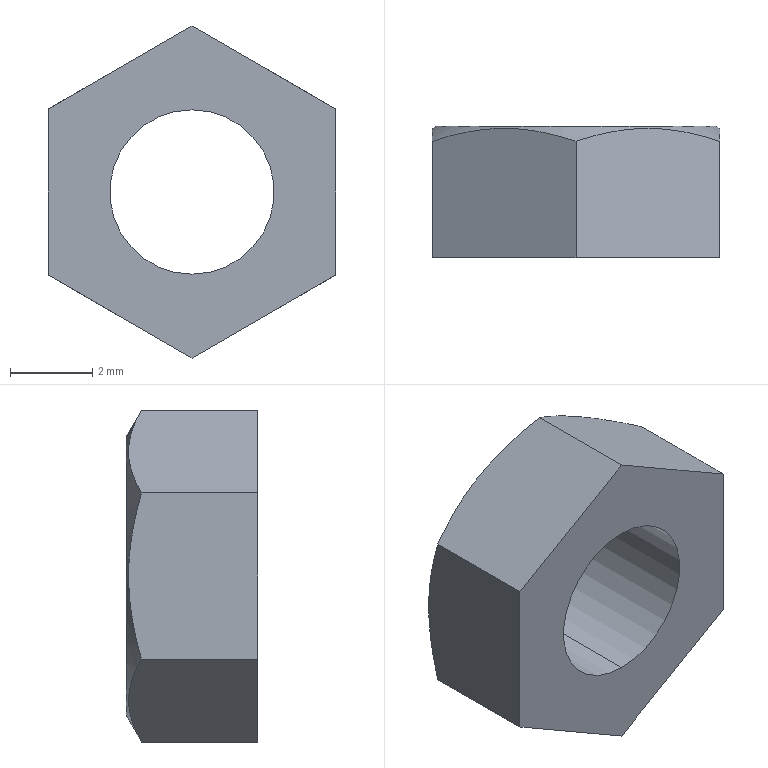Part | STEP file | NN42-M4 | 1 solid | 12 faces | box 7 x 3.2 x 8.083 mm | volume 94.914 mm3 | plane 8 | cylinder 2 | cone 2 | commonest cylinder face diameters 4 x2
STEP:
#1=CARTESIAN_POINT('',(0.,0.,0.));
#2=DIRECTION('',(0.,0.,1.));
#3=DIRECTION('',(1.,0.,0.));
#4=AXIS2_PLACEMENT_3D('',#1,#2,#3);
#5=CARTESIAN_POINT('',(0.,3.2,-2.));
#6=VERTEX_POINT('',#5);
#7=CARTESIAN_POINT('',(0.,0.,-2.));
#8=VERTEX_POINT('',#7);
#9=CARTESIAN_POINT('',(0.,3.2,-2.));
#10=DIRECTION('',(0.,-1.,0.));
#11=VECTOR('',#10,1.);
#12=LINE('',#9,#11);
#13=CARTESIAN_POINT('',(0.,3.2,0.));
#14=DIRECTION('',(0.,-1.,0.));
#15=DIRECTION('',(0.,0.,-1.));
#16=AXIS2_PLACEMENT_3D('',#13,#14,#15);
#17=CYLINDRICAL_SURFACE('',#16,2.);
#18=CARTESIAN_POINT('',(6.283,0.));
#19=DIRECTION('',(0.,1.));
#20=VECTOR('',#19,1.);
#21=LINE('',#18,#20);
#22=(GEOMETRIC_REPRESENTATION_CONTEXT(2)PARAMETRIC_REPRESENTATION_CONTEXT()REPRESENTATION_CONTEXT('',''));
#23=DEFINITIONAL_REPRESENTATION('',(#21),#22);
#24=PCURVE('',#17,#23);
#25=CARTESIAN_POINT('',(0.,3.2,0.));
#26=DIRECTION('',(0.,-1.,0.));
#27=DIRECTION('',(0.,0.,-1.));
#28=AXIS2_PLACEMENT_3D('',#25,#26,#27);
#29=CYLINDRICAL_SURFACE('',#28,2.);
#30=CARTESIAN_POINT('',(0.,0.));
#31=DIRECTION('',(0.,1.));
#32=VECTOR('',#31,1.);
#33=LINE('',#30,#32);
#34=(GEOMETRIC_REPRESENTATION_CONTEXT(2)PARAMETRIC_REPRESENTATION_CONTEXT()REPRESENTATION_CONTEXT('',''));
#35=DEFINITIONAL_REPRESENTATION('',(#33),#34);
#36=PCURVE('',#29,#35);
#37=SURFACE_CURVE('',#12,(#24,#36),.PCURVE_S1.);
#38=EDGE_CURVE('',#6,#8,#37,.T.);
#39=ORIENTED_EDGE('',*,*,#38,.T.);
#40=CARTESIAN_POINT('',(0.,0.,2.));
#41=VERTEX_POINT('',#40);
#42=CARTESIAN_POINT('',(0.,0.,0.));
#43=DIRECTION('',(0.,1.,0.));
#44=DIRECTION('',(0.,0.,1.));
#45=AXIS2_PLACEMENT_3D('',#42,#43,#44);
#46=CIRCLE('',#45,2.);
#47=CARTESIAN_POINT('',(9.425,3.2));
#48=DIRECTION('',(-1.,0.));
#49=VECTOR('',#48,1.);
#50=LINE('',#47,#49);
#51=(GEOMETRIC_REPRESENTATION_CONTEXT(2)PARAMETRIC_REPRESENTATION_CONTEXT()REPRESENTATION_CONTEXT('',''));
#52=DEFINITIONAL_REPRESENTATION('',(#50),#51);
#53=PCURVE('',#17,#52);
#54=CARTESIAN_POINT('',(0.,0.,0.));
#55=DIRECTION('',(0.,-1.,0.));
#56=DIRECTION('',(0.,0.,1.));
#57=AXIS2_PLACEMENT_3D('',#54,#55,#56);
#58=PLANE('',#57);
#59=CARTESIAN_POINT('',(2.,0.));
#60=CARTESIAN_POINT('',(2.,-3.464));
#61=CARTESIAN_POINT('',(-1.,-1.732));
#62=CARTESIAN_POINT('',(-4.,0.));
#63=CARTESIAN_POINT('',(-1.,1.732));
#64=CARTESIAN_POINT('',(2.,3.464));
#65=CARTESIAN_POINT('',(2.,0.));
#66=(BOUNDED_CURVE()B_SPLINE_CURVE(2,(#59,#60,#61,#62,#63,#64,#65),.UNSPECIFIED.,.T.,.F.)B_SPLINE_CURVE_WITH_KNOTS((1,2,2,2,2,1),(-2.094,0.,2.094,4.189,6.283,8.378),.UNSPECIFIED.)CURVE()GEOMETRIC_REPRESENTATION_ITEM()RATIONAL_B_SPLINE_CURVE((1.,0.5,1.,0.5,1.,0.5,1.))REPRESENTATION_ITEM(''));
#67=(GEOMETRIC_REPRESENTATION_CONTEXT(2)PARAMETRIC_REPRESENTATION_CONTEXT()REPRESENTATION_CONTEXT('',''));
#68=DEFINITIONAL_REPRESENTATION('',(#66),#67);
#69=PCURVE('',#58,#68);
#70=SURFACE_CURVE('',#46,(#53,#69),.PCURVE_S1.);
#71=EDGE_CURVE('',#8,#41,#70,.T.);
#72=ORIENTED_EDGE('',*,*,#71,.T.);
#73=CARTESIAN_POINT('',(0.,3.2,2.));
#74=VERTEX_POINT('',#73);
#75=CARTESIAN_POINT('',(0.,3.2,2.));
#76=DIRECTION('',(0.,-1.,0.));
#77=VECTOR('',#76,1.);
#78=LINE('',#75,#77);
#79=CARTESIAN_POINT('',(3.142,0.));
#80=DIRECTION('',(0.,1.));
#81=VECTOR('',#80,1.);
#82=LINE('',#79,#81);
#83=(GEOMETRIC_REPRESENTATION_CONTEXT(2)PARAMETRIC_REPRESENTATION_CONTEXT()REPRESENTATION_CONTEXT('',''));
#84=DEFINITIONAL_REPRESENTATION('',(#82),#83);
#85=PCURVE('',#17,#84);
#86=CARTESIAN_POINT('',(3.142,0.));
#87=DIRECTION('',(0.,1.));
#88=VECTOR('',#87,1.);
#89=LINE('',#86,#88);
#90=(GEOMETRIC_REPRESENTATION_CONTEXT(2)PARAMETRIC_REPRESENTATION_CONTEXT()REPRESENTATION_CONTEXT('',''));
#91=DEFINITIONAL_REPRESENTATION('',(#89),#90);
#92=PCURVE('',#29,#91);
#93=SURFACE_CURVE('',#78,(#85,#92),.PCURVE_S1.);
#94=EDGE_CURVE('',#74,#41,#93,.T.);
#95=ORIENTED_EDGE('',*,*,#94,.F.);
#96=CARTESIAN_POINT('',(0.,3.2,0.));
#97=DIRECTION('',(0.,-1.,0.));
#98=DIRECTION('',(0.,0.,-1.));
#99=AXIS2_PLACEMENT_3D('',#96,#97,#98);
#100=CIRCLE('',#99,2.);
#101=CARTESIAN_POINT('',(0.,0.));
#102=DIRECTION('',(1.,0.));
#103=VECTOR('',#102,1.);
#104=LINE('',#101,#103);
#105=(GEOMETRIC_REPRESENTATION_CONTEXT(2)PARAMETRIC_REPRESENTATION_CONTEXT()REPRESENTATION_CONTEXT('',''));
#106=DEFINITIONAL_REPRESENTATION('',(#104),#105);
#107=PCURVE('',#17,#106);
#108=CARTESIAN_POINT('',(0.,3.2,0.));
#109=DIRECTION('',(0.,1.,0.));
#110=DIRECTION('',(-1.,0.,0.));
#111=AXIS2_PLACEMENT_3D('',#108,#109,#110);
#112=PLANE('',#111);
#113=CARTESIAN_POINT('',(0.,-2.));
#114=CARTESIAN_POINT('',(-3.464,-2.));
#115=CARTESIAN_POINT('',(-1.732,1.));
#116=CARTESIAN_POINT('',(0.,4.));
#117=CARTESIAN_POINT('',(1.732,1.));
#118=CARTESIAN_POINT('',(3.464,-2.));
#119=CARTESIAN_POINT('',(0.,-2.));
#120=(BOUNDED_CURVE()B_SPLINE_CURVE(2,(#113,#114,#115,#116,#117,#118,#119),.UNSPECIFIED.,.T.,.F.)B_SPLINE_CURVE_WITH_KNOTS((1,2,2,2,2,1),(-2.094,0.,2.094,4.189,6.283,8.378),.UNSPECIFIED.)CURVE()GEOMETRIC_REPRESENTATION_ITEM()RATIONAL_B_SPLINE_CURVE((1.,0.5,1.,0.5,1.,0.5,1.))REPRESENTATION_ITEM(''));
#121=(GEOMETRIC_REPRESENTATION_CONTEXT(2)PARAMETRIC_REPRESENTATION_CONTEXT()REPRESENTATION_CONTEXT('',''));
#122=DEFINITIONAL_REPRESENTATION('',(#120),#121);
#123=PCURVE('',#112,#122);
#124=SURFACE_CURVE('',#100,(#107,#123),.PCURVE_S1.);
#125=EDGE_CURVE('',#74,#6,#124,.T.);
#126=ORIENTED_EDGE('',*,*,#125,.T.);
#127=EDGE_LOOP('',(#39,#72,#95,#126));
#128=FACE_BOUND('',#127,.F.);
#129=ADVANCED_FACE('',(#128),#17,.F.);
#130=CARTESIAN_POINT('',(3.4,3.2,0.));
#131=VERTEX_POINT('',#130);
#132=CARTESIAN_POINT('',(-3.4,3.2,0.));
#133=VERTEX_POINT('',#132);
#134=CARTESIAN_POINT('',(0.,3.2,0.));
#135=DIRECTION('',(0.,-1.,0.));
#136=DIRECTION('',(1.,0.,0.));
#137=AXIS2_PLACEMENT_3D('',#134,#135,#136);
#138=CIRCLE('',#137,3.4);
#139=CARTESIAN_POINT('',(0.,3.2,0.));
#140=DIRECTION('',(0.,-1.,0.));
#141=DIRECTION('',(1.,0.,0.));
#142=AXIS2_PLACEMENT_3D('',#139,#140,#141);
#143=CONICAL_SURFACE('',#142,3.4,1.047);
#144=CARTESIAN_POINT('',(0.,0.));
#145=DIRECTION('',(1.,0.));
#146=VECTOR('',#145,1.);
#147=LINE('',#144,#146);
#148=(GEOMETRIC_REPRESENTATION_CONTEXT(2)PARAMETRIC_REPRESENTATION_CONTEXT()REPRESENTATION_CONTEXT('',''));
#149=DEFINITIONAL_REPRESENTATION('',(#147),#148);
#150=PCURVE('',#143,#149);
#151=CARTESIAN_POINT('',(-3.4,0.));
#152=CARTESIAN_POINT('',(-3.4,5.889));
#153=CARTESIAN_POINT('',(1.7,2.944));
#154=CARTESIAN_POINT('',(6.8,0.));
#155=CARTESIAN_POINT('',(1.7,-2.944));
#156=CARTESIAN_POINT('',(-3.4,-5.889));
#157=CARTESIAN_POINT('',(-3.4,0.));
#158=(BOUNDED_CURVE()B_SPLINE_CURVE(2,(#151,#152,#153,#154,#155,#156,#157),.UNSPECIFIED.,.T.,.F.)B_SPLINE_CURVE_WITH_KNOTS((1,2,2,2,2,1),(-2.094,0.,2.094,4.189,6.283,8.378),.UNSPECIFIED.)CURVE()GEOMETRIC_REPRESENTATION_ITEM()RATIONAL_B_SPLINE_CURVE((1.,0.5,1.,0.5,1.,0.5,1.))REPRESENTATION_ITEM(''));
#159=(GEOMETRIC_REPRESENTATION_CONTEXT(2)PARAMETRIC_REPRESENTATION_CONTEXT()REPRESENTATION_CONTEXT('',''));
#160=DEFINITIONAL_REPRESENTATION('',(#158),#159);
#161=PCURVE('',#112,#160);
#162=SURFACE_CURVE('',#138,(#150,#161),.PCURVE_S1.);
#163=EDGE_CURVE('',#131,#133,#162,.T.);
#164=ORIENTED_EDGE('',*,*,#163,.T.);
#165=CARTESIAN_POINT('',(-3.5,3.142,0.));
#166=VERTEX_POINT('',#165);
#167=CARTESIAN_POINT('',(-3.4,3.2,0.));
#168=DIRECTION('',(-0.866,-0.5,0.));
#169=VECTOR('',#168,1.);
#170=LINE('',#167,#169);
#171=CARTESIAN_POINT('',(3.142,0.));
#172=DIRECTION('',(0.,1.));
#173=VECTOR('',#172,1.);
#174=LINE('',#171,#173);
#175=(GEOMETRIC_REPRESENTATION_CONTEXT(2)PARAMETRIC_REPRESENTATION_CONTEXT()REPRESENTATION_CONTEXT('',''));
#176=DEFINITIONAL_REPRESENTATION('',(#174),#175);
#177=PCURVE('',#143,#176);
#178=CARTESIAN_POINT('',(0.,3.2,0.));
#179=DIRECTION('',(0.,-1.,0.));
#180=DIRECTION('',(1.,0.,0.));
#181=AXIS2_PLACEMENT_3D('',#178,#179,#180);
#182=CONICAL_SURFACE('',#181,3.4,1.047);
#183=CARTESIAN_POINT('',(3.142,0.));
#184=DIRECTION('',(0.,1.));
#185=VECTOR('',#184,1.);
#186=LINE('',#183,#185);
#187=(GEOMETRIC_REPRESENTATION_CONTEXT(2)PARAMETRIC_REPRESENTATION_CONTEXT()REPRESENTATION_CONTEXT('',''));
#188=DEFINITIONAL_REPRESENTATION('',(#186),#187);
#189=PCURVE('',#182,#188);
#190=SURFACE_CURVE('',#170,(#177,#189),.PCURVE_S1.);
#191=EDGE_CURVE('',#133,#166,#190,.T.);
#192=ORIENTED_EDGE('',*,*,#191,.T.);
#193=CARTESIAN_POINT('',(-3.5,2.83,2.021));
#194=VERTEX_POINT('',#193);
#195=CARTESIAN_POINT('',(-3.5,2.83,2.021));
#196=CARTESIAN_POINT('',(-3.5,3.02,1.362));
#197=CARTESIAN_POINT('',(-3.5,3.142,0.6921));
#198=CARTESIAN_POINT('',(-3.5,3.142,0.));
#199=B_SPLINE_CURVE_WITH_KNOTS('',3,(#195,#196,#197,#198),.UNSPECIFIED.,.F.,.F.,(4,4),(0.004408,0.006464),.PIECEWISE_BEZIER_KNOTS.);
#200=CARTESIAN_POINT('',(2.618,0.3703));
#201=CARTESIAN_POINT('',(2.624,0.3617));
#202=CARTESIAN_POINT('',(2.637,0.3447));
#203=CARTESIAN_POINT('',(2.657,0.3201));
#204=CARTESIAN_POINT('',(2.678,0.2963));
#205=CARTESIAN_POINT('',(2.699,0.2735));
#206=CARTESIAN_POINT('',(2.72,0.2516));
#207=CARTESIAN_POINT('',(2.742,0.2307));
#208=CARTESIAN_POINT('',(2.764,0.2108));
#209=CARTESIAN_POINT('',(2.787,0.192));
#210=CARTESIAN_POINT('',(2.81,0.1743));
#211=CARTESIAN_POINT('',(2.833,0.1577));
#212=CARTESIAN_POINT('',(2.857,0.1422));
#213=CARTESIAN_POINT('',(2.882,0.1279));
#214=CARTESIAN_POINT('',(2.906,0.1149));
#215=CARTESIAN_POINT('',(2.931,0.1031));
#216=CARTESIAN_POINT('',(2.957,0.09264));
#217=CARTESIAN_POINT('',(2.982,0.08345));
#218=CARTESIAN_POINT('',(3.008,0.07562));
#219=CARTESIAN_POINT('',(3.035,0.06915));
#220=CARTESIAN_POINT('',(3.061,0.06408));
#221=CARTESIAN_POINT('',(3.088,0.06043));
#222=CARTESIAN_POINT('',(3.115,0.05823));
#223=CARTESIAN_POINT('',(3.133,0.05773));
#224=CARTESIAN_POINT('',(3.142,0.05774));
#225=B_SPLINE_CURVE_WITH_KNOTS('',3,(#200,#201,#202,#203,#204,#205,#206,#207,#208,#209,#210,#211,#212,#213,#214,#215,#216,#217,#218,#219,#220,#221,#222,#223,#224),.UNSPECIFIED.,.F.,.F.,(4,1,1,1,1,1,1,1,1,1,1,1,1,1,1,1,1,1,1,1,1,1,4),(0.004408,0.004502,0.004595,0.004689,0.004782,0.004875,0.004969,0.005062,0.005156,0.005249,0.005343,0.005436,0.00553,0.005623,0.005716,0.00581,0.005903,0.005997,0.00609,0.006184,0.006277,0.006371,0.006464),.QUASI_UNIFORM_KNOTS.);
#226=(GEOMETRIC_REPRESENTATION_CONTEXT(2)PARAMETRIC_REPRESENTATION_CONTEXT()REPRESENTATION_CONTEXT('',''));
#227=DEFINITIONAL_REPRESENTATION('',(#225),#226);
#228=PCURVE('',#143,#227);
#229=CARTESIAN_POINT('',(-3.5,2.83,2.021));
#230=DIRECTION('',(1.,0.,0.));
#231=DIRECTION('',(0.,0.,1.));
#232=AXIS2_PLACEMENT_3D('',#229,#230,#231);
#233=PLANE('',#232);
#234=CARTESIAN_POINT('',(0.,0.));
#235=CARTESIAN_POINT('',(-0.6583,-0.19));
#236=CARTESIAN_POINT('',(-1.329,-0.3126));
#237=CARTESIAN_POINT('',(-2.021,-0.3126));
#238=B_SPLINE_CURVE_WITH_KNOTS('',3,(#234,#235,#236,#237),.UNSPECIFIED.,.F.,.F.,(4,4),(0.004408,0.006464),.PIECEWISE_BEZIER_KNOTS.);
#239=(GEOMETRIC_REPRESENTATION_CONTEXT(2)PARAMETRIC_REPRESENTATION_CONTEXT()REPRESENTATION_CONTEXT('',''));
#240=DEFINITIONAL_REPRESENTATION('',(#238),#239);
#241=PCURVE('',#233,#240);
#242=SURFACE_CURVE('',#199,(#228,#241),.PCURVE_S1.);
#243=EDGE_CURVE('',#194,#166,#242,.T.);
#244=ORIENTED_EDGE('',*,*,#243,.F.);
#245=CARTESIAN_POINT('',(0.,2.83,4.041));
#246=VERTEX_POINT('',#245);
#247=CARTESIAN_POINT('',(0.,2.83,4.041));
#248=CARTESIAN_POINT('',(-0.5715,3.02,3.712));
#249=CARTESIAN_POINT('',(-1.152,3.142,3.377));
#250=CARTESIAN_POINT('',(-2.044,3.142,2.861));
#251=CARTESIAN_POINT('',(-2.341,3.113,2.69));
#252=CARTESIAN_POINT('',(-2.925,3.004,2.352));
#253=CARTESIAN_POINT('',(-3.214,2.925,2.186));
#254=CARTESIAN_POINT('',(-3.5,2.83,2.021));
#255=B_SPLINE_CURVE_WITH_KNOTS('',3,(#247,#248,#249,#250,#251,#252,#253,#254),.UNSPECIFIED.,.F.,.F.,(4,2,2,4),(0.000000238,0.002041,0.003061,0.004082),.UNSPECIFIED.);
#256=CARTESIAN_POINT('',(1.571,0.3703));
#257=CARTESIAN_POINT('',(1.584,0.353));
#258=CARTESIAN_POINT('',(1.61,0.3195));
#259=CARTESIAN_POINT('',(1.651,0.2728));
#260=CARTESIAN_POINT('',(1.694,0.23));
#261=CARTESIAN_POINT('',(1.739,0.1913));
#262=CARTESIAN_POINT('',(1.786,0.157));
#263=CARTESIAN_POINT('',(1.834,0.1273));
#264=CARTESIAN_POINT('',(1.884,0.1025));
#265=CARTESIAN_POINT('',(1.935,0.08287));
#266=CARTESIAN_POINT('',(1.987,0.06856));
#267=CARTESIAN_POINT('',(2.04,0.05981));
#268=CARTESIAN_POINT('',(2.093,0.05676));
#269=CARTESIAN_POINT('',(2.147,0.05956));
#270=CARTESIAN_POINT('',(2.2,0.06812));
#271=CARTESIAN_POINT('',(2.252,0.08231));
#272=CARTESIAN_POINT('',(2.304,0.1019));
#273=CARTESIAN_POINT('',(2.354,0.1267));
#274=CARTESIAN_POINT('',(2.402,0.1565));
#275=CARTESIAN_POINT('',(2.449,0.1909));
#276=CARTESIAN_POINT('',(2.494,0.2297));
#277=CARTESIAN_POINT('',(2.537,0.2726));
#278=CARTESIAN_POINT('',(2.579,0.3194));
#279=CARTESIAN_POINT('',(2.605,0.353));
#280=CARTESIAN_POINT('',(2.618,0.3703));
#281=B_SPLINE_CURVE_WITH_KNOTS('',3,(#256,#257,#258,#259,#260,#261,#262,#263,#264,#265,#266,#267,#268,#269,#270,#271,#272,#273,#274,#275,#276,#277,#278,#279,#280),.UNSPECIFIED.,.F.,.F.,(4,1,1,1,1,1,1,1,1,1,1,1,1,1,1,1,1,1,1,1,1,1,4),(0.000000238,0.0001858,0.0003713,0.0005568,0.0007424,0.0009279,0.001113,0.001299,0.001484,0.00167,0.001856,0.002041,0.002227,0.002412,0.002598,0.002783,0.002969,0.003154,0.00334,0.003525,0.003711,0.003896,0.004082),.QUASI_UNIFORM_KNOTS.);
#282=(GEOMETRIC_REPRESENTATION_CONTEXT(2)PARAMETRIC_REPRESENTATION_CONTEXT()REPRESENTATION_CONTEXT('',''));
#283=DEFINITIONAL_REPRESENTATION('',(#281),#282);
#284=PCURVE('',#143,#283);
#285=CARTESIAN_POINT('',(0.,2.83,4.041));
#286=DIRECTION('',(0.5,0.,-0.866));
#287=DIRECTION('',(0.866,0.,0.5));
#288=AXIS2_PLACEMENT_3D('',#285,#286,#287);
#289=PLANE('',#288);
#290=CARTESIAN_POINT('',(0.,0.));
#291=CARTESIAN_POINT('',(-0.6599,-0.1905));
#292=CARTESIAN_POINT('',(-1.33,-0.3122));
#293=CARTESIAN_POINT('',(-2.36,-0.3128));
#294=CARTESIAN_POINT('',(-2.704,-0.283));
#295=CARTESIAN_POINT('',(-3.378,-0.1741));
#296=CARTESIAN_POINT('',(-3.711,-0.09537));
#297=CARTESIAN_POINT('',(-4.041,0.));
#298=B_SPLINE_CURVE_WITH_KNOTS('',3,(#290,#291,#292,#293,#294,#295,#296,#297),.UNSPECIFIED.,.F.,.F.,(4,2,2,4),(0.000000238,0.002041,0.003061,0.004082),.UNSPECIFIED.);
#299=(GEOMETRIC_REPRESENTATION_CONTEXT(2)PARAMETRIC_REPRESENTATION_CONTEXT()REPRESENTATION_CONTEXT('',''));
#300=DEFINITIONAL_REPRESENTATION('',(#298),#299);
#301=PCURVE('',#289,#300);
#302=SURFACE_CURVE('',#255,(#284,#301),.PCURVE_S1.);
#303=EDGE_CURVE('',#246,#194,#302,.T.);
#304=ORIENTED_EDGE('',*,*,#303,.F.);
#305=CARTESIAN_POINT('',(3.5,2.83,2.021));
#306=VERTEX_POINT('',#305);
#307=CARTESIAN_POINT('',(3.5,2.83,2.021));
#308=CARTESIAN_POINT('',(2.929,3.02,2.351));
#309=CARTESIAN_POINT('',(2.348,3.142,2.686));
#310=CARTESIAN_POINT('',(1.456,3.142,3.201));
#311=CARTESIAN_POINT('',(1.159,3.113,3.373));
#312=CARTESIAN_POINT('',(0.5746,3.004,3.71));
#313=CARTESIAN_POINT('',(0.2861,2.925,3.876));
#314=CARTESIAN_POINT('',(0.,2.83,4.041));
#315=B_SPLINE_CURVE_WITH_KNOTS('',3,(#307,#308,#309,#310,#311,#312,#313,#314),.UNSPECIFIED.,.F.,.F.,(4,2,2,4),(0.000000238,0.002041,0.003061,0.004082),.UNSPECIFIED.);
#316=CARTESIAN_POINT('',(0.5236,0.3703));
#317=CARTESIAN_POINT('',(0.5365,0.353));
#318=CARTESIAN_POINT('',(0.5628,0.3195));
#319=CARTESIAN_POINT('',(0.6041,0.2728));
#320=CARTESIAN_POINT('',(0.6472,0.23));
#321=CARTESIAN_POINT('',(0.6921,0.1913));
#322=CARTESIAN_POINT('',(0.7388,0.157));
#323=CARTESIAN_POINT('',(0.787,0.1273));
#324=CARTESIAN_POINT('',(0.8367,0.1025));
#325=CARTESIAN_POINT('',(0.8877,0.08287));
#326=CARTESIAN_POINT('',(0.9398,0.06856));
#327=CARTESIAN_POINT('',(0.9926,0.05981));
#328=CARTESIAN_POINT('',(1.046,0.05676));
#329=CARTESIAN_POINT('',(1.1,0.05956));
#330=CARTESIAN_POINT('',(1.153,0.06812));
#331=CARTESIAN_POINT('',(1.205,0.08231));
#332=CARTESIAN_POINT('',(1.257,0.1019));
#333=CARTESIAN_POINT('',(1.307,0.1267));
#334=CARTESIAN_POINT('',(1.355,0.1565));
#335=CARTESIAN_POINT('',(1.402,0.1909));
#336=CARTESIAN_POINT('',(1.447,0.2297));
#337=CARTESIAN_POINT('',(1.49,0.2726));
#338=CARTESIAN_POINT('',(1.532,0.3194));
#339=CARTESIAN_POINT('',(1.558,0.353));
#340=CARTESIAN_POINT('',(1.571,0.3703));
#341=B_SPLINE_CURVE_WITH_KNOTS('',3,(#316,#317,#318,#319,#320,#321,#322,#323,#324,#325,#326,#327,#328,#329,#330,#331,#332,#333,#334,#335,#336,#337,#338,#339,#340),.UNSPECIFIED.,.F.,.F.,(4,1,1,1,1,1,1,1,1,1,1,1,1,1,1,1,1,1,1,1,1,1,4),(0.000000238,0.0001858,0.0003713,0.0005568,0.0007424,0.0009279,0.001113,0.001299,0.001484,0.00167,0.001856,0.002041,0.002227,0.002412,0.002598,0.002783,0.002969,0.003154,0.00334,0.003525,0.003711,0.003896,0.004082),.QUASI_UNIFORM_KNOTS.);
#342=(GEOMETRIC_REPRESENTATION_CONTEXT(2)PARAMETRIC_REPRESENTATION_CONTEXT()REPRESENTATION_CONTEXT('',''));
#343=DEFINITIONAL_REPRESENTATION('',(#341),#342);
#344=PCURVE('',#143,#343);
#345=CARTESIAN_POINT('',(3.5,2.83,2.021));
#346=DIRECTION('',(-0.5,0.,-0.866));
#347=DIRECTION('',(0.866,0.,-0.5));
#348=AXIS2_PLACEMENT_3D('',#345,#346,#347);
#349=PLANE('',#348);
#350=CARTESIAN_POINT('',(0.,0.));
#351=CARTESIAN_POINT('',(-0.6599,-0.1905));
#352=CARTESIAN_POINT('',(-1.33,-0.3122));
#353=CARTESIAN_POINT('',(-2.36,-0.3128));
#354=CARTESIAN_POINT('',(-2.704,-0.283));
#355=CARTESIAN_POINT('',(-3.378,-0.1741));
#356=CARTESIAN_POINT('',(-3.711,-0.09537));
#357=CARTESIAN_POINT('',(-4.041,0.));
#358=B_SPLINE_CURVE_WITH_KNOTS('',3,(#350,#351,#352,#353,#354,#355,#356,#357),.UNSPECIFIED.,.F.,.F.,(4,2,2,4),(0.000000238,0.002041,0.003061,0.004082),.UNSPECIFIED.);
#359=(GEOMETRIC_REPRESENTATION_CONTEXT(2)PARAMETRIC_REPRESENTATION_CONTEXT()REPRESENTATION_CONTEXT('',''));
#360=DEFINITIONAL_REPRESENTATION('',(#358),#359);
#361=PCURVE('',#349,#360);
#362=SURFACE_CURVE('',#315,(#344,#361),.PCURVE_S1.);
#363=EDGE_CURVE('',#306,#246,#362,.T.);
#364=ORIENTED_EDGE('',*,*,#363,.F.);
#365=CARTESIAN_POINT('',(3.5,3.142,0.));
#366=VERTEX_POINT('',#365);
#367=CARTESIAN_POINT('',(3.5,3.142,0.));
#368=CARTESIAN_POINT('',(3.5,3.142,0.6917));
#369=CARTESIAN_POINT('',(3.5,3.019,1.363));
#370=CARTESIAN_POINT('',(3.5,2.83,2.021));
#371=B_SPLINE_CURVE_WITH_KNOTS('',3,(#367,#368,#369,#370),.UNSPECIFIED.,.F.,.F.,(4,4),(0.006464,0.008519),.PIECEWISE_BEZIER_KNOTS.);
#372=CARTESIAN_POINT('',(0.,0.05774));
#373=CARTESIAN_POINT('',(0.008983,0.05773));
#374=CARTESIAN_POINT('',(0.02693,0.05823));
#375=CARTESIAN_POINT('',(0.05373,0.06043));
#376=CARTESIAN_POINT('',(0.08039,0.06408));
#377=CARTESIAN_POINT('',(0.1069,0.06915));
#378=CARTESIAN_POINT('',(0.1331,0.07562));
#379=CARTESIAN_POINT('',(0.1591,0.08346));
#380=CARTESIAN_POINT('',(0.1849,0.09265));
#381=CARTESIAN_POINT('',(0.2103,0.1031));
#382=CARTESIAN_POINT('',(0.2354,0.1149));
#383=CARTESIAN_POINT('',(0.2601,0.128));
#384=CARTESIAN_POINT('',(0.2845,0.1422));
#385=CARTESIAN_POINT('',(0.3084,0.1577));
#386=CARTESIAN_POINT('',(0.332,0.1743));
#387=CARTESIAN_POINT('',(0.3551,0.1921));
#388=CARTESIAN_POINT('',(0.3778,0.2109));
#389=CARTESIAN_POINT('',(0.4,0.2308));
#390=CARTESIAN_POINT('',(0.4218,0.2516));
#391=CARTESIAN_POINT('',(0.4431,0.2735));
#392=CARTESIAN_POINT('',(0.4639,0.2964));
#393=CARTESIAN_POINT('',(0.4843,0.3201));
#394=CARTESIAN_POINT('',(0.5042,0.3447));
#395=CARTESIAN_POINT('',(0.5172,0.3617));
#396=CARTESIAN_POINT('',(0.5236,0.3703));
#397=B_SPLINE_CURVE_WITH_KNOTS('',3,(#372,#373,#374,#375,#376,#377,#378,#379,#380,#381,#382,#383,#384,#385,#386,#387,#388,#389,#390,#391,#392,#393,#394,#395,#396),.UNSPECIFIED.,.F.,.F.,(4,1,1,1,1,1,1,1,1,1,1,1,1,1,1,1,1,1,1,1,1,1,4),(0.006464,0.006557,0.006651,0.006744,0.006838,0.006931,0.007024,0.007118,0.007211,0.007305,0.007398,0.007491,0.007585,0.007678,0.007772,0.007865,0.007958,0.008052,0.008145,0.008239,0.008332,0.008425,0.008519),.QUASI_UNIFORM_KNOTS.);
#398=(GEOMETRIC_REPRESENTATION_CONTEXT(2)PARAMETRIC_REPRESENTATION_CONTEXT()REPRESENTATION_CONTEXT('',''));
#399=DEFINITIONAL_REPRESENTATION('',(#397),#398);
#400=PCURVE('',#143,#399);
#401=CARTESIAN_POINT('',(3.5,2.83,-2.021));
#402=DIRECTION('',(-1.,0.,0.));
#403=DIRECTION('',(0.,0.,-1.));
#404=AXIS2_PLACEMENT_3D('',#401,#402,#403);
#405=PLANE('',#404);
#406=CARTESIAN_POINT('',(-2.021,-0.3126));
#407=CARTESIAN_POINT('',(-2.712,-0.3126));
#408=CARTESIAN_POINT('',(-3.384,-0.1898));
#409=CARTESIAN_POINT('',(-4.041,0.));
#410=B_SPLINE_CURVE_WITH_KNOTS('',3,(#406,#407,#408,#409),.UNSPECIFIED.,.F.,.F.,(4,4),(0.006464,0.008519),.PIECEWISE_BEZIER_KNOTS.);
#411=(GEOMETRIC_REPRESENTATION_CONTEXT(2)PARAMETRIC_REPRESENTATION_CONTEXT()REPRESENTATION_CONTEXT('',''));
#412=DEFINITIONAL_REPRESENTATION('',(#410),#411);
#413=PCURVE('',#405,#412);
#414=SURFACE_CURVE('',#371,(#400,#413),.PCURVE_S1.);
#415=EDGE_CURVE('',#366,#306,#414,.T.);
#416=ORIENTED_EDGE('',*,*,#415,.F.);
#417=CARTESIAN_POINT('',(3.4,3.2,0.));
#418=DIRECTION('',(0.866,-0.5,0.));
#419=VECTOR('',#418,1.);
#420=LINE('',#417,#419);
#421=CARTESIAN_POINT('',(0.,0.));
#422=DIRECTION('',(0.,1.));
#423=VECTOR('',#422,1.);
#424=LINE('',#421,#423);
#425=(GEOMETRIC_REPRESENTATION_CONTEXT(2)PARAMETRIC_REPRESENTATION_CONTEXT()REPRESENTATION_CONTEXT('',''));
#426=DEFINITIONAL_REPRESENTATION('',(#424),#425);
#427=PCURVE('',#143,#426);
#428=CARTESIAN_POINT('',(6.283,0.));
#429=DIRECTION('',(0.,1.));
#430=VECTOR('',#429,1.);
#431=LINE('',#428,#430);
#432=(GEOMETRIC_REPRESENTATION_CONTEXT(2)PARAMETRIC_REPRESENTATION_CONTEXT()REPRESENTATION_CONTEXT('',''));
#433=DEFINITIONAL_REPRESENTATION('',(#431),#432);
#434=PCURVE('',#182,#433);
#435=SURFACE_CURVE('',#420,(#427,#434),.PCURVE_S1.);
#436=EDGE_CURVE('',#131,#366,#435,.T.);
#437=ORIENTED_EDGE('',*,*,#436,.F.);
#438=EDGE_LOOP('',(#164,#192,#244,#304,#364,#416,#437));
#439=FACE_BOUND('',#438,.T.);
#440=ADVANCED_FACE('',(#439),#143,.T.);
#441=ORIENTED_EDGE('',*,*,#191,.F.);
#442=CARTESIAN_POINT('',(0.,3.2,0.));
#443=DIRECTION('',(0.,-1.,0.));
#444=DIRECTION('',(1.,0.,0.));
#445=AXIS2_PLACEMENT_3D('',#442,#443,#444);
#446=CIRCLE('',#445,3.4);
#447=CARTESIAN_POINT('',(0.,0.));
#448=DIRECTION('',(1.,0.));
#449=VECTOR('',#448,1.);
#450=LINE('',#447,#449);
#451=(GEOMETRIC_REPRESENTATION_CONTEXT(2)PARAMETRIC_REPRESENTATION_CONTEXT()REPRESENTATION_CONTEXT('',''));
#452=DEFINITIONAL_REPRESENTATION('',(#450),#451);
#453=PCURVE('',#182,#452);
#454=CARTESIAN_POINT('',(-3.4,0.));
#455=CARTESIAN_POINT('',(-3.4,5.889));
#456=CARTESIAN_POINT('',(1.7,2.944));
#457=CARTESIAN_POINT('',(6.8,0.));
#458=CARTESIAN_POINT('',(1.7,-2.944));
#459=CARTESIAN_POINT('',(-3.4,-5.889));
#460=CARTESIAN_POINT('',(-3.4,0.));
#461=(BOUNDED_CURVE()B_SPLINE_CURVE(2,(#454,#455,#456,#457,#458,#459,#460),.UNSPECIFIED.,.T.,.F.)B_SPLINE_CURVE_WITH_KNOTS((1,2,2,2,2,1),(-2.094,0.,2.094,4.189,6.283,8.378),.UNSPECIFIED.)CURVE()GEOMETRIC_REPRESENTATION_ITEM()RATIONAL_B_SPLINE_CURVE((1.,0.5,1.,0.5,1.,0.5,1.))REPRESENTATION_ITEM(''));
#462=(GEOMETRIC_REPRESENTATION_CONTEXT(2)PARAMETRIC_REPRESENTATION_CONTEXT()REPRESENTATION_CONTEXT('',''));
#463=DEFINITIONAL_REPRESENTATION('',(#461),#462);
#464=PCURVE('',#112,#463);
#465=SURFACE_CURVE('',#446,(#453,#464),.PCURVE_S1.);
#466=EDGE_CURVE('',#133,#131,#465,.T.);
#467=ORIENTED_EDGE('',*,*,#466,.T.);
#468=ORIENTED_EDGE('',*,*,#436,.T.);
#469=CARTESIAN_POINT('',(3.5,2.83,-2.021));
#470=VERTEX_POINT('',#469);
#471=CARTESIAN_POINT('',(3.5,2.83,-2.021));
#472=CARTESIAN_POINT('',(3.5,3.02,-1.362));
#473=CARTESIAN_POINT('',(3.5,3.142,-0.6921));
#474=CARTESIAN_POINT('',(3.5,3.142,0.));
#475=B_SPLINE_CURVE_WITH_KNOTS('',3,(#471,#472,#473,#474),.UNSPECIFIED.,.F.,.F.,(4,4),(0.004408,0.006464),.PIECEWISE_BEZIER_KNOTS.);
#476=CARTESIAN_POINT('',(5.76,0.3703));
#477=CARTESIAN_POINT('',(5.766,0.3617));
#478=CARTESIAN_POINT('',(5.779,0.3447));
#479=CARTESIAN_POINT('',(5.799,0.3201));
#480=CARTESIAN_POINT('',(5.819,0.2963));
#481=CARTESIAN_POINT('',(5.84,0.2735));
#482=CARTESIAN_POINT('',(5.861,0.2516));
#483=CARTESIAN_POINT('',(5.883,0.2307));
#484=CARTESIAN_POINT('',(5.905,0.2108));
#485=CARTESIAN_POINT('',(5.928,0.192));
#486=CARTESIAN_POINT('',(5.951,0.1743));
#487=CARTESIAN_POINT('',(5.975,0.1577));
#488=CARTESIAN_POINT('',(5.999,0.1422));
#489=CARTESIAN_POINT('',(6.023,0.1279));
#490=CARTESIAN_POINT('',(6.048,0.1149));
#491=CARTESIAN_POINT('',(6.073,0.1031));
#492=CARTESIAN_POINT('',(6.098,0.09264));
#493=CARTESIAN_POINT('',(6.124,0.08345));
#494=CARTESIAN_POINT('',(6.15,0.07562));
#495=CARTESIAN_POINT('',(6.176,0.06915));
#496=CARTESIAN_POINT('',(6.203,0.06408));
#497=CARTESIAN_POINT('',(6.229,0.06043));
#498=CARTESIAN_POINT('',(6.256,0.05823));
#499=CARTESIAN_POINT('',(6.274,0.05773));
#500=CARTESIAN_POINT('',(6.283,0.05774));
#501=B_SPLINE_CURVE_WITH_KNOTS('',3,(#476,#477,#478,#479,#480,#481,#482,#483,#484,#485,#486,#487,#488,#489,#490,#491,#492,#493,#494,#495,#496,#497,#498,#499,#500),.UNSPECIFIED.,.F.,.F.,(4,1,1,1,1,1,1,1,1,1,1,1,1,1,1,1,1,1,1,1,1,1,4),(0.004408,0.004502,0.004595,0.004689,0.004782,0.004875,0.004969,0.005062,0.005156,0.005249,0.005343,0.005436,0.00553,0.005623,0.005716,0.00581,0.005903,0.005997,0.00609,0.006184,0.006277,0.006371,0.006464),.QUASI_UNIFORM_KNOTS.);
#502=(GEOMETRIC_REPRESENTATION_CONTEXT(2)PARAMETRIC_REPRESENTATION_CONTEXT()REPRESENTATION_CONTEXT('',''));
#503=DEFINITIONAL_REPRESENTATION('',(#501),#502);
#504=PCURVE('',#182,#503);
#505=CARTESIAN_POINT('',(0.,0.));
#506=CARTESIAN_POINT('',(-0.6583,-0.19));
#507=CARTESIAN_POINT('',(-1.329,-0.3126));
#508=CARTESIAN_POINT('',(-2.021,-0.3126));
#509=B_SPLINE_CURVE_WITH_KNOTS('',3,(#505,#506,#507,#508),.UNSPECIFIED.,.F.,.F.,(4,4),(0.004408,0.006464),.PIECEWISE_BEZIER_KNOTS.);
#510=(GEOMETRIC_REPRESENTATION_CONTEXT(2)PARAMETRIC_REPRESENTATION_CONTEXT()REPRESENTATION_CONTEXT('',''));
#511=DEFINITIONAL_REPRESENTATION('',(#509),#510);
#512=PCURVE('',#405,#511);
#513=SURFACE_CURVE('',#475,(#504,#512),.PCURVE_S1.);
#514=EDGE_CURVE('',#470,#366,#513,.T.);
#515=ORIENTED_EDGE('',*,*,#514,.F.);
#516=CARTESIAN_POINT('',(0.,2.83,-4.041));
#517=VERTEX_POINT('',#516);
#518=CARTESIAN_POINT('',(0.,2.83,-4.041));
#519=CARTESIAN_POINT('',(0.5715,3.02,-3.712));
#520=CARTESIAN_POINT('',(1.152,3.142,-3.377));
#521=CARTESIAN_POINT('',(2.044,3.142,-2.861));
#522=CARTESIAN_POINT('',(2.341,3.113,-2.69));
#523=CARTESIAN_POINT('',(2.925,3.004,-2.352));
#524=CARTESIAN_POINT('',(3.214,2.925,-2.186));
#525=CARTESIAN_POINT('',(3.5,2.83,-2.021));
#526=B_SPLINE_CURVE_WITH_KNOTS('',3,(#518,#519,#520,#521,#522,#523,#524,#525),.UNSPECIFIED.,.F.,.F.,(4,2,2,4),(0.000000238,0.002041,0.003061,0.004082),.UNSPECIFIED.);
#527=CARTESIAN_POINT('',(4.712,0.3703));
#528=CARTESIAN_POINT('',(4.725,0.353));
#529=CARTESIAN_POINT('',(4.752,0.3195));
#530=CARTESIAN_POINT('',(4.793,0.2728));
#531=CARTESIAN_POINT('',(4.836,0.23));
#532=CARTESIAN_POINT('',(4.881,0.1913));
#533=CARTESIAN_POINT('',(4.928,0.157));
#534=CARTESIAN_POINT('',(4.976,0.1273));
#535=CARTESIAN_POINT('',(5.026,0.1025));
#536=CARTESIAN_POINT('',(5.076,0.08287));
#537=CARTESIAN_POINT('',(5.129,0.06856));
#538=CARTESIAN_POINT('',(5.181,0.05981));
#539=CARTESIAN_POINT('',(5.235,0.05676));
#540=CARTESIAN_POINT('',(5.288,0.05956));
#541=CARTESIAN_POINT('',(5.342,0.06812));
#542=CARTESIAN_POINT('',(5.394,0.08231));
#543=CARTESIAN_POINT('',(5.445,0.1019));
#544=CARTESIAN_POINT('',(5.495,0.1267));
#545=CARTESIAN_POINT('',(5.544,0.1565));
#546=CARTESIAN_POINT('',(5.591,0.1909));
#547=CARTESIAN_POINT('',(5.636,0.2297));
#548=CARTESIAN_POINT('',(5.679,0.2726));
#549=CARTESIAN_POINT('',(5.72,0.3194));
#550=CARTESIAN_POINT('',(5.747,0.353));
#551=CARTESIAN_POINT('',(5.76,0.3703));
#552=B_SPLINE_CURVE_WITH_KNOTS('',3,(#527,#528,#529,#530,#531,#532,#533,#534,#535,#536,#537,#538,#539,#540,#541,#542,#543,#544,#545,#546,#547,#548,#549,#550,#551),.UNSPECIFIED.,.F.,.F.,(4,1,1,1,1,1,1,1,1,1,1,1,1,1,1,1,1,1,1,1,1,1,4),(0.000000238,0.0001858,0.0003713,0.0005568,0.0007424,0.0009279,0.001113,0.001299,0.001484,0.00167,0.001856,0.002041,0.002227,0.002412,0.002598,0.002783,0.002969,0.003154,0.00334,0.003525,0.003711,0.003896,0.004082),.QUASI_UNIFORM_KNOTS.);
#553=(GEOMETRIC_REPRESENTATION_CONTEXT(2)PARAMETRIC_REPRESENTATION_CONTEXT()REPRESENTATION_CONTEXT('',''));
#554=DEFINITIONAL_REPRESENTATION('',(#552),#553);
#555=PCURVE('',#182,#554);
#556=CARTESIAN_POINT('',(0.,2.83,-4.041));
#557=DIRECTION('',(-0.5,0.,0.866));
#558=DIRECTION('',(-0.866,0.,-0.5));
#559=AXIS2_PLACEMENT_3D('',#556,#557,#558);
#560=PLANE('',#559);
#561=CARTESIAN_POINT('',(0.,0.));
#562=CARTESIAN_POINT('',(-0.6599,-0.1905));
#563=CARTESIAN_POINT('',(-1.33,-0.3122));
#564=CARTESIAN_POINT('',(-2.36,-0.3128));
#565=CARTESIAN_POINT('',(-2.704,-0.283));
#566=CARTESIAN_POINT('',(-3.378,-0.1741));
#567=CARTESIAN_POINT('',(-3.711,-0.09537));
#568=CARTESIAN_POINT('',(-4.041,0.));
#569=B_SPLINE_CURVE_WITH_KNOTS('',3,(#561,#562,#563,#564,#565,#566,#567,#568),.UNSPECIFIED.,.F.,.F.,(4,2,2,4),(0.000000238,0.002041,0.003061,0.004082),.UNSPECIFIED.);
#570=(GEOMETRIC_REPRESENTATION_CONTEXT(2)PARAMETRIC_REPRESENTATION_CONTEXT()REPRESENTATION_CONTEXT('',''));
#571=DEFINITIONAL_REPRESENTATION('',(#569),#570);
#572=PCURVE('',#560,#571);
#573=SURFACE_CURVE('',#526,(#555,#572),.PCURVE_S1.);
#574=EDGE_CURVE('',#517,#470,#573,.T.);
#575=ORIENTED_EDGE('',*,*,#574,.F.);
#576=CARTESIAN_POINT('',(-3.5,2.83,-2.021));
#577=VERTEX_POINT('',#576);
#578=CARTESIAN_POINT('',(-3.5,2.83,-2.021));
#579=CARTESIAN_POINT('',(-2.929,3.02,-2.351));
#580=CARTESIAN_POINT('',(-2.348,3.142,-2.686));
#581=CARTESIAN_POINT('',(-1.456,3.142,-3.201));
#582=CARTESIAN_POINT('',(-1.159,3.113,-3.373));
#583=CARTESIAN_POINT('',(-0.5746,3.004,-3.71));
#584=CARTESIAN_POINT('',(-0.2861,2.925,-3.876));
#585=CARTESIAN_POINT('',(0.,2.83,-4.041));
#586=B_SPLINE_CURVE_WITH_KNOTS('',3,(#578,#579,#580,#581,#582,#583,#584,#585),.UNSPECIFIED.,.F.,.F.,(4,2,2,4),(0.000000238,0.002041,0.003061,0.004082),.UNSPECIFIED.);
#587=CARTESIAN_POINT('',(3.665,0.3703));
#588=CARTESIAN_POINT('',(3.678,0.353));
#589=CARTESIAN_POINT('',(3.704,0.3195));
#590=CARTESIAN_POINT('',(3.746,0.2728));
#591=CARTESIAN_POINT('',(3.789,0.23));
#592=CARTESIAN_POINT('',(3.834,0.1913));
#593=CARTESIAN_POINT('',(3.88,0.157));
#594=CARTESIAN_POINT('',(3.929,0.1273));
#595=CARTESIAN_POINT('',(3.978,0.1025));
#596=CARTESIAN_POINT('',(4.029,0.08287));
#597=CARTESIAN_POINT('',(4.081,0.06856));
#598=CARTESIAN_POINT('',(4.134,0.05981));
#599=CARTESIAN_POINT('',(4.188,0.05676));
#600=CARTESIAN_POINT('',(4.241,0.05956));
#601=CARTESIAN_POINT('',(4.294,0.06812));
#602=CARTESIAN_POINT('',(4.347,0.08231));
#603=CARTESIAN_POINT('',(4.398,0.1019));
#604=CARTESIAN_POINT('',(4.448,0.1267));
#605=CARTESIAN_POINT('',(4.497,0.1565));
#606=CARTESIAN_POINT('',(4.543,0.1909));
#607=CARTESIAN_POINT('',(4.589,0.2297));
#608=CARTESIAN_POINT('',(4.632,0.2726));
#609=CARTESIAN_POINT('',(4.673,0.3194));
#610=CARTESIAN_POINT('',(4.7,0.353));
#611=CARTESIAN_POINT('',(4.712,0.3703));
#612=B_SPLINE_CURVE_WITH_KNOTS('',3,(#587,#588,#589,#590,#591,#592,#593,#594,#595,#596,#597,#598,#599,#600,#601,#602,#603,#604,#605,#606,#607,#608,#609,#610,#611),.UNSPECIFIED.,.F.,.F.,(4,1,1,1,1,1,1,1,1,1,1,1,1,1,1,1,1,1,1,1,1,1,4),(0.000000238,0.0001858,0.0003713,0.0005568,0.0007424,0.0009279,0.001113,0.001299,0.001484,0.00167,0.001856,0.002041,0.002227,0.002412,0.002598,0.002783,0.002969,0.003154,0.00334,0.003525,0.003711,0.003896,0.004082),.QUASI_UNIFORM_KNOTS.);
#613=(GEOMETRIC_REPRESENTATION_CONTEXT(2)PARAMETRIC_REPRESENTATION_CONTEXT()REPRESENTATION_CONTEXT('',''));
#614=DEFINITIONAL_REPRESENTATION('',(#612),#613);
#615=PCURVE('',#182,#614);
#616=CARTESIAN_POINT('',(-3.5,2.83,-2.021));
#617=DIRECTION('',(0.5,0.,0.866));
#618=DIRECTION('',(-0.866,0.,0.5));
#619=AXIS2_PLACEMENT_3D('',#616,#617,#618);
#620=PLANE('',#619);
#621=CARTESIAN_POINT('',(0.,0.));
#622=CARTESIAN_POINT('',(-0.6599,-0.1905));
#623=CARTESIAN_POINT('',(-1.33,-0.3122));
#624=CARTESIAN_POINT('',(-2.36,-0.3128));
#625=CARTESIAN_POINT('',(-2.704,-0.283));
#626=CARTESIAN_POINT('',(-3.378,-0.1741));
#627=CARTESIAN_POINT('',(-3.711,-0.09537));
#628=CARTESIAN_POINT('',(-4.041,0.));
#629=B_SPLINE_CURVE_WITH_KNOTS('',3,(#621,#622,#623,#624,#625,#626,#627,#628),.UNSPECIFIED.,.F.,.F.,(4,2,2,4),(0.000000238,0.002041,0.003061,0.004082),.UNSPECIFIED.);
#630=(GEOMETRIC_REPRESENTATION_CONTEXT(2)PARAMETRIC_REPRESENTATION_CONTEXT()REPRESENTATION_CONTEXT('',''));
#631=DEFINITIONAL_REPRESENTATION('',(#629),#630);
#632=PCURVE('',#620,#631);
#633=SURFACE_CURVE('',#586,(#615,#632),.PCURVE_S1.);
#634=EDGE_CURVE('',#577,#517,#633,.T.);
#635=ORIENTED_EDGE('',*,*,#634,.F.);
#636=CARTESIAN_POINT('',(-3.5,3.142,0.));
#637=CARTESIAN_POINT('',(-3.5,3.142,-0.6917));
#638=CARTESIAN_POINT('',(-3.5,3.019,-1.363));
#639=CARTESIAN_POINT('',(-3.5,2.83,-2.021));
#640=B_SPLINE_CURVE_WITH_KNOTS('',3,(#636,#637,#638,#639),.UNSPECIFIED.,.F.,.F.,(4,4),(0.006464,0.008519),.PIECEWISE_BEZIER_KNOTS.);
#641=CARTESIAN_POINT('',(3.142,0.05774));
#642=CARTESIAN_POINT('',(3.151,0.05773));
#643=CARTESIAN_POINT('',(3.169,0.05823));
#644=CARTESIAN_POINT('',(3.195,0.06043));
#645=CARTESIAN_POINT('',(3.222,0.06408));
#646=CARTESIAN_POINT('',(3.248,0.06915));
#647=CARTESIAN_POINT('',(3.275,0.07562));
#648=CARTESIAN_POINT('',(3.301,0.08346));
#649=CARTESIAN_POINT('',(3.326,0.09265));
#650=CARTESIAN_POINT('',(3.352,0.1031));
#651=CARTESIAN_POINT('',(3.377,0.1149));
#652=CARTESIAN_POINT('',(3.402,0.128));
#653=CARTESIAN_POINT('',(3.426,0.1422));
#654=CARTESIAN_POINT('',(3.45,0.1577));
#655=CARTESIAN_POINT('',(3.474,0.1743));
#656=CARTESIAN_POINT('',(3.497,0.1921));
#657=CARTESIAN_POINT('',(3.519,0.2109));
#658=CARTESIAN_POINT('',(3.542,0.2308));
#659=CARTESIAN_POINT('',(3.563,0.2516));
#660=CARTESIAN_POINT('',(3.585,0.2735));
#661=CARTESIAN_POINT('',(3.606,0.2964));
#662=CARTESIAN_POINT('',(3.626,0.3201));
#663=CARTESIAN_POINT('',(3.646,0.3447));
#664=CARTESIAN_POINT('',(3.659,0.3617));
#665=CARTESIAN_POINT('',(3.665,0.3703));
#666=B_SPLINE_CURVE_WITH_KNOTS('',3,(#641,#642,#643,#644,#645,#646,#647,#648,#649,#650,#651,#652,#653,#654,#655,#656,#657,#658,#659,#660,#661,#662,#663,#664,#665),.UNSPECIFIED.,.F.,.F.,(4,1,1,1,1,1,1,1,1,1,1,1,1,1,1,1,1,1,1,1,1,1,4),(0.006464,0.006557,0.006651,0.006744,0.006838,0.006931,0.007024,0.007118,0.007211,0.007305,0.007398,0.007491,0.007585,0.007678,0.007772,0.007865,0.007958,0.008052,0.008145,0.008239,0.008332,0.008425,0.008519),.QUASI_UNIFORM_KNOTS.);
#667=(GEOMETRIC_REPRESENTATION_CONTEXT(2)PARAMETRIC_REPRESENTATION_CONTEXT()REPRESENTATION_CONTEXT('',''));
#668=DEFINITIONAL_REPRESENTATION('',(#666),#667);
#669=PCURVE('',#182,#668);
#670=CARTESIAN_POINT('',(-2.021,-0.3126));
#671=CARTESIAN_POINT('',(-2.712,-0.3126));
#672=CARTESIAN_POINT('',(-3.384,-0.1898));
#673=CARTESIAN_POINT('',(-4.041,0.));
#674=B_SPLINE_CURVE_WITH_KNOTS('',3,(#670,#671,#672,#673),.UNSPECIFIED.,.F.,.F.,(4,4),(0.006464,0.008519),.PIECEWISE_BEZIER_KNOTS.);
#675=(GEOMETRIC_REPRESENTATION_CONTEXT(2)PARAMETRIC_REPRESENTATION_CONTEXT()REPRESENTATION_CONTEXT('',''));
#676=DEFINITIONAL_REPRESENTATION('',(#674),#675);
#677=PCURVE('',#233,#676);
#678=SURFACE_CURVE('',#640,(#669,#677),.PCURVE_S1.);
#679=EDGE_CURVE('',#166,#577,#678,.T.);
#680=ORIENTED_EDGE('',*,*,#679,.F.);
#681=EDGE_LOOP('',(#441,#467,#468,#515,#575,#635,#680));
#682=FACE_BOUND('',#681,.T.);
#683=ADVANCED_FACE('',(#682),#182,.T.);
#684=CARTESIAN_POINT('',(0.,3.2,0.));
#685=DIRECTION('',(0.,-1.,0.));
#686=DIRECTION('',(0.,0.,-1.));
#687=AXIS2_PLACEMENT_3D('',#684,#685,#686);
#688=CIRCLE('',#687,2.);
#689=CARTESIAN_POINT('',(0.,-2.));
#690=CARTESIAN_POINT('',(-3.464,-2.));
#691=CARTESIAN_POINT('',(-1.732,1.));
#692=CARTESIAN_POINT('',(0.,4.));
#693=CARTESIAN_POINT('',(1.732,1.));
#694=CARTESIAN_POINT('',(3.464,-2.));
#695=CARTESIAN_POINT('',(0.,-2.));
#696=(BOUNDED_CURVE()B_SPLINE_CURVE(2,(#689,#690,#691,#692,#693,#694,#695),.UNSPECIFIED.,.T.,.F.)B_SPLINE_CURVE_WITH_KNOTS((1,2,2,2,2,1),(-2.094,0.,2.094,4.189,6.283,8.378),.UNSPECIFIED.)CURVE()GEOMETRIC_REPRESENTATION_ITEM()RATIONAL_B_SPLINE_CURVE((1.,0.5,1.,0.5,1.,0.5,1.))REPRESENTATION_ITEM(''));
#697=(GEOMETRIC_REPRESENTATION_CONTEXT(2)PARAMETRIC_REPRESENTATION_CONTEXT()REPRESENTATION_CONTEXT('',''));
#698=DEFINITIONAL_REPRESENTATION('',(#696),#697);
#699=PCURVE('',#112,#698);
#700=CARTESIAN_POINT('',(0.,0.));
#701=DIRECTION('',(1.,0.));
#702=VECTOR('',#701,1.);
#703=LINE('',#700,#702);
#704=(GEOMETRIC_REPRESENTATION_CONTEXT(2)PARAMETRIC_REPRESENTATION_CONTEXT()REPRESENTATION_CONTEXT('',''));
#705=DEFINITIONAL_REPRESENTATION('',(#703),#704);
#706=PCURVE('',#29,#705);
#707=SURFACE_CURVE('',#688,(#699,#706),.PCURVE_S1.);
#708=EDGE_CURVE('',#6,#74,#707,.T.);
#709=ORIENTED_EDGE('',*,*,#708,.T.);
#710=ORIENTED_EDGE('',*,*,#125,.T.);
#711=EDGE_LOOP('',(#709,#710));
#712=FACE_BOUND('',#711,.T.);
#713=ORIENTED_EDGE('',*,*,#163,.F.);
#714=ORIENTED_EDGE('',*,*,#466,.F.);
#715=EDGE_LOOP('',(#713,#714));
#716=FACE_BOUND('',#715,.T.);
#717=ADVANCED_FACE('',(#712,#716),#112,.T.);
#718=ORIENTED_EDGE('',*,*,#514,.T.);
#719=ORIENTED_EDGE('',*,*,#415,.T.);
#720=CARTESIAN_POINT('',(3.5,0.,2.021));
#721=VERTEX_POINT('',#720);
#722=CARTESIAN_POINT('',(3.5,0.,2.021));
#723=DIRECTION('',(0.,1.,0.));
#724=VECTOR('',#723,1.);
#725=LINE('',#722,#724);
#726=CARTESIAN_POINT('',(-4.041,2.83));
#727=DIRECTION('',(0.,-1.));
#728=VECTOR('',#727,1.);
#729=LINE('',#726,#728);
#730=(GEOMETRIC_REPRESENTATION_CONTEXT(2)PARAMETRIC_REPRESENTATION_CONTEXT()REPRESENTATION_CONTEXT('',''));
#731=DEFINITIONAL_REPRESENTATION('',(#729),#730);
#732=PCURVE('',#405,#731);
#733=CARTESIAN_POINT('',(0.,2.83));
#734=DIRECTION('',(0.,-1.));
#735=VECTOR('',#734,1.);
#736=LINE('',#733,#735);
#737=(GEOMETRIC_REPRESENTATION_CONTEXT(2)PARAMETRIC_REPRESENTATION_CONTEXT()REPRESENTATION_CONTEXT('',''));
#738=DEFINITIONAL_REPRESENTATION('',(#736),#737);
#739=PCURVE('',#349,#738);
#740=SURFACE_CURVE('',#725,(#732,#739),.PCURVE_S1.);
#741=EDGE_CURVE('',#721,#306,#740,.T.);
#742=ORIENTED_EDGE('',*,*,#741,.F.);
#743=CARTESIAN_POINT('',(3.5,0.,-2.021));
#744=VERTEX_POINT('',#743);
#745=CARTESIAN_POINT('',(3.5,0.,-2.021));
#746=DIRECTION('',(0.,0.,1.));
#747=VECTOR('',#746,1.);
#748=LINE('',#745,#747);
#749=CARTESIAN_POINT('',(0.,2.83));
#750=DIRECTION('',(-1.,0.));
#751=VECTOR('',#750,1.);
#752=LINE('',#749,#751);
#753=(GEOMETRIC_REPRESENTATION_CONTEXT(2)PARAMETRIC_REPRESENTATION_CONTEXT()REPRESENTATION_CONTEXT('',''));
#754=DEFINITIONAL_REPRESENTATION('',(#752),#753);
#755=PCURVE('',#405,#754);
#756=CARTESIAN_POINT('',(-2.021,-3.5));
#757=DIRECTION('',(1.,0.));
#758=VECTOR('',#757,1.);
#759=LINE('',#756,#758);
#760=(GEOMETRIC_REPRESENTATION_CONTEXT(2)PARAMETRIC_REPRESENTATION_CONTEXT()REPRESENTATION_CONTEXT('',''));
#761=DEFINITIONAL_REPRESENTATION('',(#759),#760);
#762=PCURVE('',#58,#761);
#763=SURFACE_CURVE('',#748,(#755,#762),.PCURVE_S1.);
#764=EDGE_CURVE('',#744,#721,#763,.T.);
#765=ORIENTED_EDGE('',*,*,#764,.F.);
#766=CARTESIAN_POINT('',(3.5,0.,-2.021));
#767=DIRECTION('',(0.,1.,0.));
#768=VECTOR('',#767,1.);
#769=LINE('',#766,#768);
#770=CARTESIAN_POINT('',(0.,2.83));
#771=DIRECTION('',(0.,-1.));
#772=VECTOR('',#771,1.);
#773=LINE('',#770,#772);
#774=(GEOMETRIC_REPRESENTATION_CONTEXT(2)PARAMETRIC_REPRESENTATION_CONTEXT()REPRESENTATION_CONTEXT('',''));
#775=DEFINITIONAL_REPRESENTATION('',(#773),#774);
#776=PCURVE('',#405,#775);
#777=CARTESIAN_POINT('',(-4.041,2.83));
#778=DIRECTION('',(0.,-1.));
#779=VECTOR('',#778,1.);
#780=LINE('',#777,#779);
#781=(GEOMETRIC_REPRESENTATION_CONTEXT(2)PARAMETRIC_REPRESENTATION_CONTEXT()REPRESENTATION_CONTEXT('',''));
#782=DEFINITIONAL_REPRESENTATION('',(#780),#781);
#783=PCURVE('',#560,#782);
#784=SURFACE_CURVE('',#769,(#776,#783),.PCURVE_S1.);
#785=EDGE_CURVE('',#744,#470,#784,.T.);
#786=ORIENTED_EDGE('',*,*,#785,.T.);
#787=EDGE_LOOP('',(#718,#719,#742,#765,#786));
#788=FACE_BOUND('',#787,.T.);
#789=ADVANCED_FACE('',(#788),#405,.F.);
#790=ORIENTED_EDGE('',*,*,#574,.T.);
#791=ORIENTED_EDGE('',*,*,#785,.F.);
#792=CARTESIAN_POINT('',(0.,0.,-4.041));
#793=VERTEX_POINT('',#792);
#794=CARTESIAN_POINT('',(0.,0.,-4.041));
#795=DIRECTION('',(0.866,0.,0.5));
#796=VECTOR('',#795,1.);
#797=LINE('',#794,#796);
#798=CARTESIAN_POINT('',(0.,2.83));
#799=DIRECTION('',(-1.,0.));
#800=VECTOR('',#799,1.);
#801=LINE('',#798,#800);
#802=(GEOMETRIC_REPRESENTATION_CONTEXT(2)PARAMETRIC_REPRESENTATION_CONTEXT()REPRESENTATION_CONTEXT('',''));
#803=DEFINITIONAL_REPRESENTATION('',(#801),#802);
#804=PCURVE('',#560,#803);
#805=CARTESIAN_POINT('',(-4.041,0.));
#806=DIRECTION('',(0.5,-0.866));
#807=VECTOR('',#806,1.);
#808=LINE('',#805,#807);
#809=(GEOMETRIC_REPRESENTATION_CONTEXT(2)PARAMETRIC_REPRESENTATION_CONTEXT()REPRESENTATION_CONTEXT('',''));
#810=DEFINITIONAL_REPRESENTATION('',(#808),#809);
#811=PCURVE('',#58,#810);
#812=SURFACE_CURVE('',#797,(#804,#811),.PCURVE_S1.);
#813=EDGE_CURVE('',#793,#744,#812,.T.);
#814=ORIENTED_EDGE('',*,*,#813,.F.);
#815=CARTESIAN_POINT('',(0.,0.,-4.041));
#816=DIRECTION('',(0.,1.,0.));
#817=VECTOR('',#816,1.);
#818=LINE('',#815,#817);
#819=CARTESIAN_POINT('',(0.,2.83));
#820=DIRECTION('',(0.,-1.));
#821=VECTOR('',#820,1.);
#822=LINE('',#819,#821);
#823=(GEOMETRIC_REPRESENTATION_CONTEXT(2)PARAMETRIC_REPRESENTATION_CONTEXT()REPRESENTATION_CONTEXT('',''));
#824=DEFINITIONAL_REPRESENTATION('',(#822),#823);
#825=PCURVE('',#560,#824);
#826=CARTESIAN_POINT('',(-4.041,2.83));
#827=DIRECTION('',(0.,-1.));
#828=VECTOR('',#827,1.);
#829=LINE('',#826,#828);
#830=(GEOMETRIC_REPRESENTATION_CONTEXT(2)PARAMETRIC_REPRESENTATION_CONTEXT()REPRESENTATION_CONTEXT('',''));
#831=DEFINITIONAL_REPRESENTATION('',(#829),#830);
#832=PCURVE('',#620,#831);
#833=SURFACE_CURVE('',#818,(#825,#832),.PCURVE_S1.);
#834=EDGE_CURVE('',#793,#517,#833,.T.);
#835=ORIENTED_EDGE('',*,*,#834,.T.);
#836=EDGE_LOOP('',(#790,#791,#814,#835));
#837=FACE_BOUND('',#836,.T.);
#838=ADVANCED_FACE('',(#837),#560,.F.);
#839=ORIENTED_EDGE('',*,*,#634,.T.);
#840=ORIENTED_EDGE('',*,*,#834,.F.);
#841=CARTESIAN_POINT('',(-3.5,0.,-2.021));
#842=VERTEX_POINT('',#841);
#843=CARTESIAN_POINT('',(-3.5,0.,-2.021));
#844=DIRECTION('',(0.866,0.,-0.5));
#845=VECTOR('',#844,1.);
#846=LINE('',#843,#845);
#847=CARTESIAN_POINT('',(0.,2.83));
#848=DIRECTION('',(-1.,0.));
#849=VECTOR('',#848,1.);
#850=LINE('',#847,#849);
#851=(GEOMETRIC_REPRESENTATION_CONTEXT(2)PARAMETRIC_REPRESENTATION_CONTEXT()REPRESENTATION_CONTEXT('',''));
#852=DEFINITIONAL_REPRESENTATION('',(#850),#851);
#853=PCURVE('',#620,#852);
#854=CARTESIAN_POINT('',(-2.021,3.5));
#855=DIRECTION('',(-0.5,-0.866));
#856=VECTOR('',#855,1.);
#857=LINE('',#854,#856);
#858=(GEOMETRIC_REPRESENTATION_CONTEXT(2)PARAMETRIC_REPRESENTATION_CONTEXT()REPRESENTATION_CONTEXT('',''));
#859=DEFINITIONAL_REPRESENTATION('',(#857),#858);
#860=PCURVE('',#58,#859);
#861=SURFACE_CURVE('',#846,(#853,#860),.PCURVE_S1.);
#862=EDGE_CURVE('',#842,#793,#861,.T.);
#863=ORIENTED_EDGE('',*,*,#862,.F.);
#864=CARTESIAN_POINT('',(-3.5,0.,-2.021));
#865=DIRECTION('',(0.,1.,0.));
#866=VECTOR('',#865,1.);
#867=LINE('',#864,#866);
#868=CARTESIAN_POINT('',(0.,2.83));
#869=DIRECTION('',(0.,-1.));
#870=VECTOR('',#869,1.);
#871=LINE('',#868,#870);
#872=(GEOMETRIC_REPRESENTATION_CONTEXT(2)PARAMETRIC_REPRESENTATION_CONTEXT()REPRESENTATION_CONTEXT('',''));
#873=DEFINITIONAL_REPRESENTATION('',(#871),#872);
#874=PCURVE('',#620,#873);
#875=CARTESIAN_POINT('',(-4.041,2.83));
#876=DIRECTION('',(0.,-1.));
#877=VECTOR('',#876,1.);
#878=LINE('',#875,#877);
#879=(GEOMETRIC_REPRESENTATION_CONTEXT(2)PARAMETRIC_REPRESENTATION_CONTEXT()REPRESENTATION_CONTEXT('',''));
#880=DEFINITIONAL_REPRESENTATION('',(#878),#879);
#881=PCURVE('',#233,#880);
#882=SURFACE_CURVE('',#867,(#874,#881),.PCURVE_S1.);
#883=EDGE_CURVE('',#842,#577,#882,.T.);
#884=ORIENTED_EDGE('',*,*,#883,.T.);
#885=EDGE_LOOP('',(#839,#840,#863,#884));
#886=FACE_BOUND('',#885,.T.);
#887=ADVANCED_FACE('',(#886),#620,.F.);
#888=ORIENTED_EDGE('',*,*,#243,.T.);
#889=ORIENTED_EDGE('',*,*,#679,.T.);
#890=ORIENTED_EDGE('',*,*,#883,.F.);
#891=CARTESIAN_POINT('',(-3.5,0.,2.021));
#892=VERTEX_POINT('',#891);
#893=CARTESIAN_POINT('',(-3.5,0.,2.021));
#894=DIRECTION('',(0.,0.,-1.));
#895=VECTOR('',#894,1.);
#896=LINE('',#893,#895);
#897=CARTESIAN_POINT('',(0.,2.83));
#898=DIRECTION('',(-1.,0.));
#899=VECTOR('',#898,1.);
#900=LINE('',#897,#899);
#901=(GEOMETRIC_REPRESENTATION_CONTEXT(2)PARAMETRIC_REPRESENTATION_CONTEXT()REPRESENTATION_CONTEXT('',''));
#902=DEFINITIONAL_REPRESENTATION('',(#900),#901);
#903=PCURVE('',#233,#902);
#904=CARTESIAN_POINT('',(2.021,3.5));
#905=DIRECTION('',(-1.,0.));
#906=VECTOR('',#905,1.);
#907=LINE('',#904,#906);
#908=(GEOMETRIC_REPRESENTATION_CONTEXT(2)PARAMETRIC_REPRESENTATION_CONTEXT()REPRESENTATION_CONTEXT('',''));
#909=DEFINITIONAL_REPRESENTATION('',(#907),#908);
#910=PCURVE('',#58,#909);
#911=SURFACE_CURVE('',#896,(#903,#910),.PCURVE_S1.);
#912=EDGE_CURVE('',#892,#842,#911,.T.);
#913=ORIENTED_EDGE('',*,*,#912,.F.);
#914=CARTESIAN_POINT('',(-3.5,0.,2.021));
#915=DIRECTION('',(0.,1.,0.));
#916=VECTOR('',#915,1.);
#917=LINE('',#914,#916);
#918=CARTESIAN_POINT('',(0.,2.83));
#919=DIRECTION('',(0.,-1.));
#920=VECTOR('',#919,1.);
#921=LINE('',#918,#920);
#922=(GEOMETRIC_REPRESENTATION_CONTEXT(2)PARAMETRIC_REPRESENTATION_CONTEXT()REPRESENTATION_CONTEXT('',''));
#923=DEFINITIONAL_REPRESENTATION('',(#921),#922);
#924=PCURVE('',#233,#923);
#925=CARTESIAN_POINT('',(-4.041,2.83));
#926=DIRECTION('',(0.,-1.));
#927=VECTOR('',#926,1.);
#928=LINE('',#925,#927);
#929=(GEOMETRIC_REPRESENTATION_CONTEXT(2)PARAMETRIC_REPRESENTATION_CONTEXT()REPRESENTATION_CONTEXT('',''));
#930=DEFINITIONAL_REPRESENTATION('',(#928),#929);
#931=PCURVE('',#289,#930);
#932=SURFACE_CURVE('',#917,(#924,#931),.PCURVE_S1.);
#933=EDGE_CURVE('',#892,#194,#932,.T.);
#934=ORIENTED_EDGE('',*,*,#933,.T.);
#935=EDGE_LOOP('',(#888,#889,#890,#913,#934));
#936=FACE_BOUND('',#935,.T.);
#937=ADVANCED_FACE('',(#936),#233,.F.);
#938=ORIENTED_EDGE('',*,*,#303,.T.);
#939=ORIENTED_EDGE('',*,*,#933,.F.);
#940=CARTESIAN_POINT('',(0.,0.,4.041));
#941=VERTEX_POINT('',#940);
#942=CARTESIAN_POINT('',(0.,0.,4.041));
#943=DIRECTION('',(-0.866,0.,-0.5));
#944=VECTOR('',#943,1.);
#945=LINE('',#942,#944);
#946=CARTESIAN_POINT('',(0.,2.83));
#947=DIRECTION('',(-1.,0.));
#948=VECTOR('',#947,1.);
#949=LINE('',#946,#948);
#950=(GEOMETRIC_REPRESENTATION_CONTEXT(2)PARAMETRIC_REPRESENTATION_CONTEXT()REPRESENTATION_CONTEXT('',''));
#951=DEFINITIONAL_REPRESENTATION('',(#949),#950);
#952=PCURVE('',#289,#951);
#953=CARTESIAN_POINT('',(4.041,0.));
#954=DIRECTION('',(-0.5,0.866));
#955=VECTOR('',#954,1.);
#956=LINE('',#953,#955);
#957=(GEOMETRIC_REPRESENTATION_CONTEXT(2)PARAMETRIC_REPRESENTATION_CONTEXT()REPRESENTATION_CONTEXT('',''));
#958=DEFINITIONAL_REPRESENTATION('',(#956),#957);
#959=PCURVE('',#58,#958);
#960=SURFACE_CURVE('',#945,(#952,#959),.PCURVE_S1.);
#961=EDGE_CURVE('',#941,#892,#960,.T.);
#962=ORIENTED_EDGE('',*,*,#961,.F.);
#963=CARTESIAN_POINT('',(0.,0.,4.041));
#964=DIRECTION('',(0.,1.,0.));
#965=VECTOR('',#964,1.);
#966=LINE('',#963,#965);
#967=CARTESIAN_POINT('',(0.,2.83));
#968=DIRECTION('',(0.,-1.));
#969=VECTOR('',#968,1.);
#970=LINE('',#967,#969);
#971=(GEOMETRIC_REPRESENTATION_CONTEXT(2)PARAMETRIC_REPRESENTATION_CONTEXT()REPRESENTATION_CONTEXT('',''));
#972=DEFINITIONAL_REPRESENTATION('',(#970),#971);
#973=PCURVE('',#289,#972);
#974=CARTESIAN_POINT('',(-4.041,2.83));
#975=DIRECTION('',(0.,-1.));
#976=VECTOR('',#975,1.);
#977=LINE('',#974,#976);
#978=(GEOMETRIC_REPRESENTATION_CONTEXT(2)PARAMETRIC_REPRESENTATION_CONTEXT()REPRESENTATION_CONTEXT('',''));
#979=DEFINITIONAL_REPRESENTATION('',(#977),#978);
#980=PCURVE('',#349,#979);
#981=SURFACE_CURVE('',#966,(#973,#980),.PCURVE_S1.);
#982=EDGE_CURVE('',#941,#246,#981,.T.);
#983=ORIENTED_EDGE('',*,*,#982,.T.);
#984=EDGE_LOOP('',(#938,#939,#962,#983));
#985=FACE_BOUND('',#984,.T.);
#986=ADVANCED_FACE('',(#985),#289,.F.);
#987=ORIENTED_EDGE('',*,*,#363,.T.);
#988=ORIENTED_EDGE('',*,*,#982,.F.);
#989=CARTESIAN_POINT('',(3.5,0.,2.021));
#990=DIRECTION('',(-0.866,0.,0.5));
#991=VECTOR('',#990,1.);
#992=LINE('',#989,#991);
#993=CARTESIAN_POINT('',(0.,2.83));
#994=DIRECTION('',(-1.,0.));
#995=VECTOR('',#994,1.);
#996=LINE('',#993,#995);
#997=(GEOMETRIC_REPRESENTATION_CONTEXT(2)PARAMETRIC_REPRESENTATION_CONTEXT()REPRESENTATION_CONTEXT('',''));
#998=DEFINITIONAL_REPRESENTATION('',(#996),#997);
#999=PCURVE('',#349,#998);
#1000=CARTESIAN_POINT('',(2.021,-3.5));
#1001=DIRECTION('',(0.5,0.866));
#1002=VECTOR('',#1001,1.);
#1003=LINE('',#1000,#1002);
#1004=(GEOMETRIC_REPRESENTATION_CONTEXT(2)PARAMETRIC_REPRESENTATION_CONTEXT()REPRESENTATION_CONTEXT('',''));
#1005=DEFINITIONAL_REPRESENTATION('',(#1003),#1004);
#1006=PCURVE('',#58,#1005);
#1007=SURFACE_CURVE('',#992,(#999,#1006),.PCURVE_S1.);
#1008=EDGE_CURVE('',#721,#941,#1007,.T.);
#1009=ORIENTED_EDGE('',*,*,#1008,.F.);
#1010=ORIENTED_EDGE('',*,*,#741,.T.);
#1011=EDGE_LOOP('',(#987,#988,#1009,#1010));
#1012=FACE_BOUND('',#1011,.T.);
#1013=ADVANCED_FACE('',(#1012),#349,.F.);
#1014=ORIENTED_EDGE('',*,*,#71,.T.);
#1015=CARTESIAN_POINT('',(0.,0.,0.));
#1016=DIRECTION('',(0.,1.,0.));
#1017=DIRECTION('',(0.,0.,1.));
#1018=AXIS2_PLACEMENT_3D('',#1015,#1016,#1017);
#1019=CIRCLE('',#1018,2.);
#1020=CARTESIAN_POINT('',(2.,0.));
#1021=CARTESIAN_POINT('',(2.,-3.464));
#1022=CARTESIAN_POINT('',(-1.,-1.732));
#1023=CARTESIAN_POINT('',(-4.,0.));
#1024=CARTESIAN_POINT('',(-1.,1.732));
#1025=CARTESIAN_POINT('',(2.,3.464));
#1026=CARTESIAN_POINT('',(2.,0.));
#1027=(BOUNDED_CURVE()B_SPLINE_CURVE(2,(#1020,#1021,#1022,#1023,#1024,#1025,#1026),.UNSPECIFIED.,.T.,.F.)B_SPLINE_CURVE_WITH_KNOTS((1,2,2,2,2,1),(-2.094,0.,2.094,4.189,6.283,8.378),.UNSPECIFIED.)CURVE()GEOMETRIC_REPRESENTATION_ITEM()RATIONAL_B_SPLINE_CURVE((1.,0.5,1.,0.5,1.,0.5,1.))REPRESENTATION_ITEM(''));
#1028=(GEOMETRIC_REPRESENTATION_CONTEXT(2)PARAMETRIC_REPRESENTATION_CONTEXT()REPRESENTATION_CONTEXT('',''));
#1029=DEFINITIONAL_REPRESENTATION('',(#1027),#1028);
#1030=PCURVE('',#58,#1029);
#1031=CARTESIAN_POINT('',(3.142,3.2));
#1032=DIRECTION('',(-1.,0.));
#1033=VECTOR('',#1032,1.);
#1034=LINE('',#1031,#1033);
#1035=(GEOMETRIC_REPRESENTATION_CONTEXT(2)PARAMETRIC_REPRESENTATION_CONTEXT()REPRESENTATION_CONTEXT('',''));
#1036=DEFINITIONAL_REPRESENTATION('',(#1034),#1035);
#1037=PCURVE('',#29,#1036);
#1038=SURFACE_CURVE('',#1019,(#1030,#1037),.PCURVE_S1.);
#1039=EDGE_CURVE('',#41,#8,#1038,.T.);
#1040=ORIENTED_EDGE('',*,*,#1039,.T.);
#1041=EDGE_LOOP('',(#1014,#1040));
#1042=FACE_BOUND('',#1041,.T.);
#1043=ORIENTED_EDGE('',*,*,#1008,.T.);
#1044=ORIENTED_EDGE('',*,*,#961,.T.);
#1045=ORIENTED_EDGE('',*,*,#912,.T.);
#1046=ORIENTED_EDGE('',*,*,#862,.T.);
#1047=ORIENTED_EDGE('',*,*,#813,.T.);
#1048=ORIENTED_EDGE('',*,*,#764,.T.);
#1049=EDGE_LOOP('',(#1043,#1044,#1045,#1046,#1047,#1048));
#1050=FACE_BOUND('',#1049,.T.);
#1051=ADVANCED_FACE('',(#1042,#1050),#58,.T.);
#1052=ORIENTED_EDGE('',*,*,#1039,.T.);
#1053=ORIENTED_EDGE('',*,*,#38,.F.);
#1054=ORIENTED_EDGE('',*,*,#708,.T.);
#1055=ORIENTED_EDGE('',*,*,#94,.T.);
#1056=EDGE_LOOP('',(#1052,#1053,#1054,#1055));
#1057=FACE_BOUND('',#1056,.F.);
#1058=ADVANCED_FACE('',(#1057),#29,.F.);
#1059=CLOSED_SHELL('',(#129,#440,#683,#717,#789,#838,#887,#937,#986,#1013,#1051,#1058));
#1060=MANIFOLD_SOLID_BREP('',#1059);
#1061=(LENGTH_UNIT()NAMED_UNIT(*)SI_UNIT(.MILLI.,.METRE.));
#1062=UNCERTAINTY_MEASURE_WITH_UNIT(LENGTH_MEASURE(0.0002),#1061,'','');
#1063=(NAMED_UNIT(*)PLANE_ANGLE_UNIT()SI_UNIT($,.RADIAN.));
#1064=(NAMED_UNIT(*)SI_UNIT($,.STERADIAN.)SOLID_ANGLE_UNIT());
#1065=(GEOMETRIC_REPRESENTATION_CONTEXT(3)GLOBAL_UNCERTAINTY_ASSIGNED_CONTEXT((#1062))GLOBAL_UNIT_ASSIGNED_CONTEXT((#1061,#1063,#1064))REPRESENTATION_CONTEXT('',''));
#1066=ADVANCED_BREP_SHAPE_REPRESENTATION('',(#4,#1060),#1065);